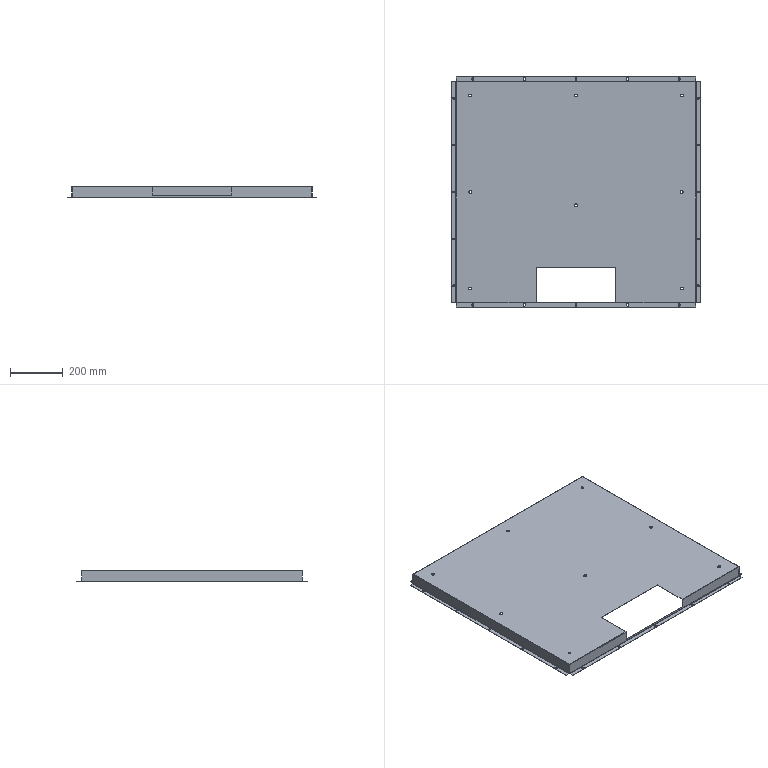Part | 1 solid | 186 faces | box 940 x 870 x 44 mm | volume 911475 mm3 | plane 94 | cylinder 84 | spline 8 | commonest cylinder face diameters 7 x50 11 x16 1 x9 3 x9